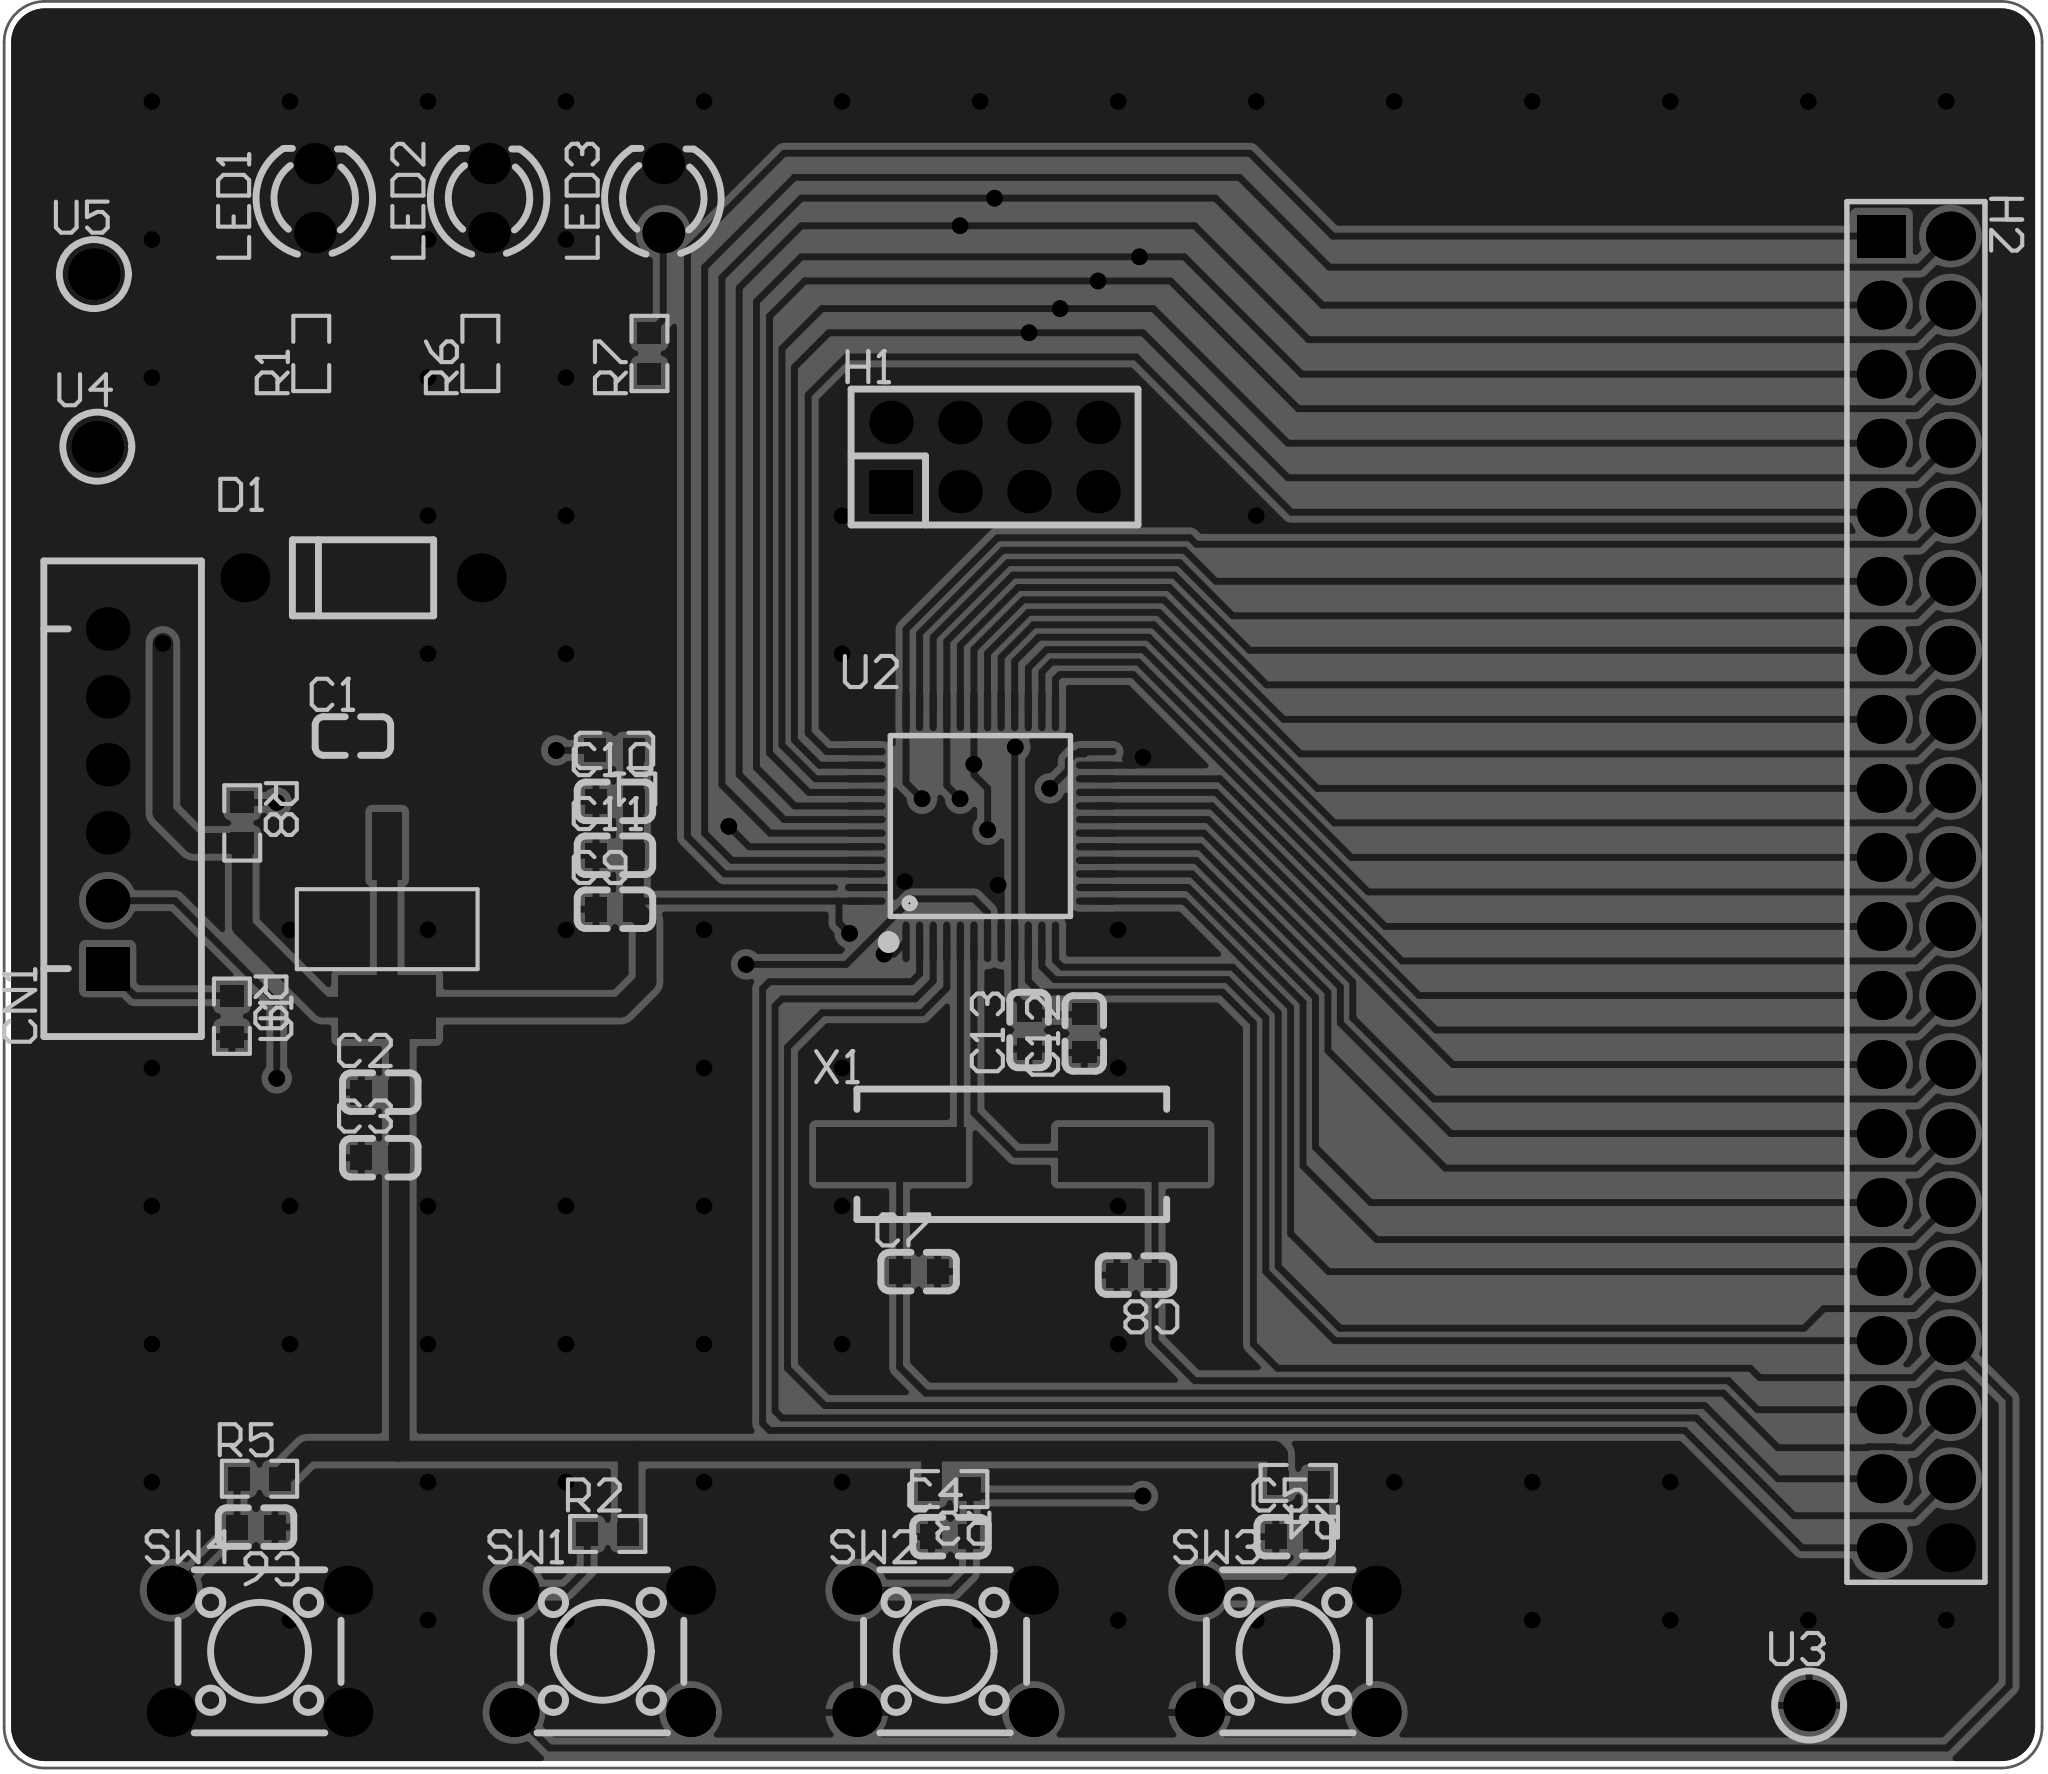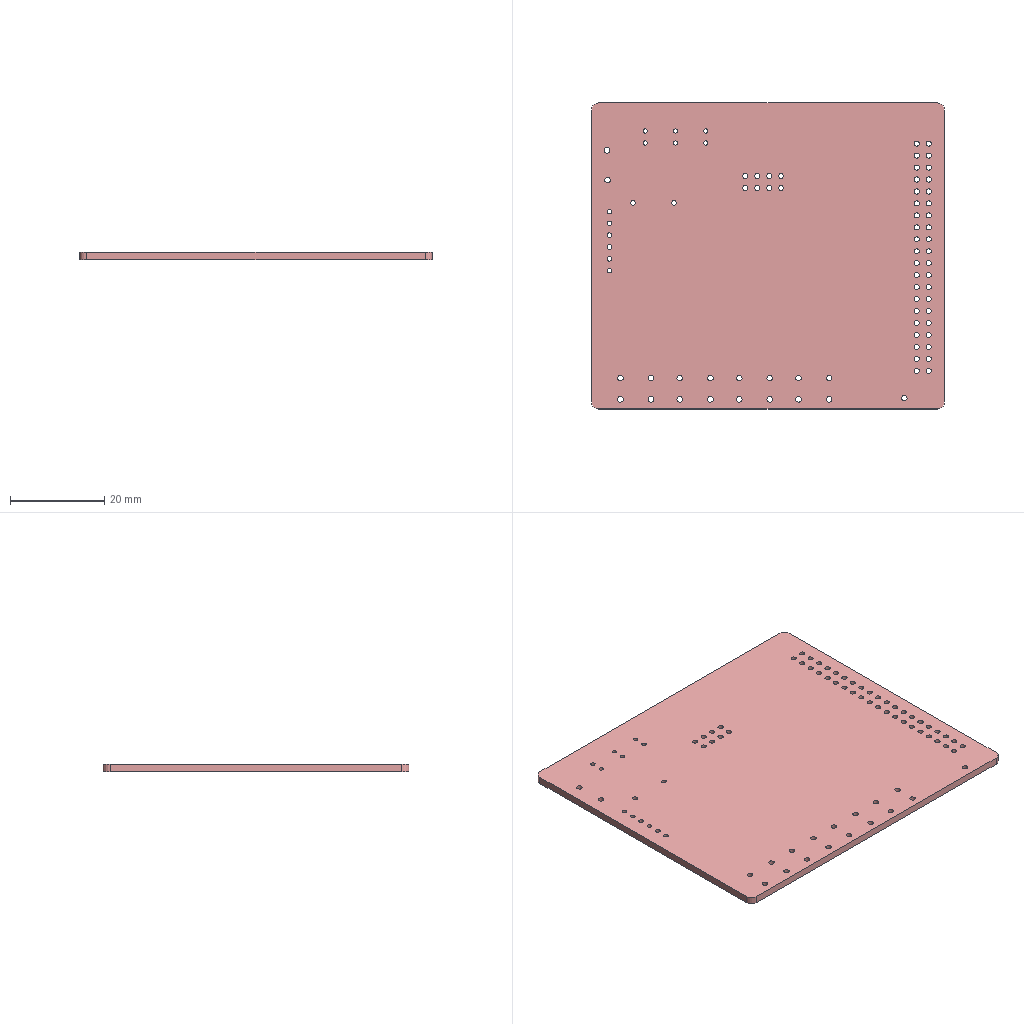Circuit board layout | Altium Designer | box 75 x 65 x 1.6 mm
Layer stack:
# Altium Designer layer stack of  (unit mm; dielectric type: 0 none, 1 core, 2 prepreg, 3 surface material)
index,name,kind,layer,copper_thickness_mm,dielectric_type,dielectric_thickness_mm,dielectric_material,dielectric_constant
0,Top Paste Mask Layer,other,,,,,,
1,Top Silkscreen Layer,other,,,,,,
2,Top Solder Mask Layer,dielectric,,,3,0.01,,3.3
3,Top Layer,copper,Top Layer,0.035,,,,
4,Dielectric1,dielectric,,,3,1.51,FR4,4.5
5,Bottom Layer,copper,Bottom Layer,0.035,,,,
6,Bottom Solder Mask Layer,dielectric,,,3,0.01,,3.3
7,Bottom Silkscreen Layer,other,,,,,,
8,Bottom Paste Mask Layer,other,,,,,,
# drill layer pairs: low layer,high layer
drill_pair,Top Layer,Bottom Layer
Part placement:
Designator,Comment,Layer,Footprint,Center-X(mm),Center-Y(mm),Rotation
C1,47uF,TopLayer,C0603,96.275,119.528,0
C2,47uF,TopLayer,C0603,97.282,106.426,0
C3,100nF,TopLayer,C0603,97.282,104.013,0
C4,100nF,TopLayer,C0603,118.266,90.07,0
C5,100nF,TopLayer,C0603,130.937,90.07,0
C6,100nF,TopLayer,C0603,92.71,90.424,180
C7,22pF,TopLayer,C0603,117.094,99.822,0
C8,22pF,TopLayer,C0603,125.095,99.695,180
C9,100nF,TopLayer,C0603,105.918,113.157,0
C10,100nF,TopLayer,C0603,105.918,117.126,0
C11,100nF,TopLayer,C0603,105.918,115.141,0
C12,1uF,TopLayer,C0603,123.19,108.585,90
C13,10nF,TopLayer,C0603,121.158,108.712,90
CN1,XH-6A,TopLayer,CONN-TH_6P-P2.50_XH-6A,87.249,117.221,90
D1,,TopLayer,DO_1N4007,96.647,125.349,0
H1,A2541HWV-2x4P,TopLayer,HDR-TH_8P-P2.54-V-F-R2-C4-S2.54-1,119.888,129.794,0
H2,2.54mm 2*20P straight pin header,TopLayer,HDR-TH_40P-P2.54-V-M-R2-C20-S2.54,153.797,113.792,270
L1,CBG160808U000T,TopLayer,L0603,105.901,118.999,180
LED1,,TopLayer,LED_TH-3mm,94.869,139.319,90
LED2,,TopLayer,LED_TH-3mm,101.282,139.319,90
LED3,,TopLayer,LED_TH-3mm,107.696,139.319,90
R1,1K,TopLayer,R0603,94.742,133.604,90
R2,10K,TopLayer,R0603,105.651,90.17,0
R3,10K,TopLayer,R0603,118.237,91.821,180
R4,10K,TopLayer,R0603,131.064,92.048,180
R5,10K,TopLayer,R0603,92.837,92.202,0
R6,330,TopLayer,R0603,100.965,133.604,90
R7,330,TopLayer,R0603,107.188,133.604,90
R8,10K,TopLayer,R0603,92.202,116.332,270
R9,10K,TopLayer,R0603,91.821,109.22,270
SW1,TS-1095-A5B2-D1,TopLayer,SW-TH_4P-L6.0-W6.0-P4.50-LS6.5,105.452,85.852,0
SW2,TS-1095-A5B2-D1,TopLayer,SW-TH_4P-L6.0-W6.0-P4.50-LS6.5,118.068,85.852,0
SW3,TS-1095-A5B2-D1,TopLayer,SW-TH_4P-L6.0-W6.0-P4.50-LS6.5,130.683,85.852,0
SW4,TS-1095-A5B2-D1,TopLayer,SW-TH_4P-L6.0-W6.0-P4.50-LS6.5,92.837,85.852,0
U1,AMS1117-3.3,TopLayer,SOT-223-3_L6.5-W3.4-P2.30-LS7.0-BR,97.536,112.522,90
U2,GD32E230C8T6,TopLayer,LQFP-48_L7.0-W7.0-P0.50-LS9.0-BL,119.38,116.205,0
U3,RH-5000,TopLayer,TEST-TH_BD2.54-P1.4_RED,149.868,83.859,0
U4,RH-5000,TopLayer,TEST-TH_BD2.54-P1.4_RED,86.868,130.175,0
U5,RH-5000,TopLayer,TEST-TH_BD2.54-P1.4_RED,86.741,136.525,0
X1,8MHz,TopLayer,CRYSTAL-SMD_L11.5-W4.8-LS12.7,120.523,104.14,0
Pad and via stacks:
# Altium Designer via and pad stacks of  (unit mm). Each distinct definition once, with the count of objects using it.
# via: kind,start_layer,end_layer,hole_mm,diameter_mm,mode(0 simple;1 top-mid-bottom;2 full stack),diameter_per_layer,count,example_net
# pad: kind,layer,hole_mm,hole_type(0 round;1 square;2 slot),plating,top_size,top_shape(1 round;2 rect;3 octagon;9 rounded rect),mid_size,bottom_size,mode,footprint,size_per_layer,count,example
pad,Top Layer,0,0,plated,0.8x0.9,2,0.8x0.9,0.8x0.9,0,C0603,,26,C1.2
pad,Top Layer,0,0,plated,0.8x0.864,2,0.8x0.864,0.8x0.864,0,L0603,,2,L1.1
pad,Top Layer,0,0,plated,0.8065x0.864,2,0.8065x0.864,0.8065x0.864,0,R0603,,18,R1.2
pad,Top Layer,0,0,plated,2.5x1.1,2,2.5x1.1,2.5x1.1,0,SOT-223-3_L6.5-W3.4-P2.30-LS7.0-BR,,3,U1.1
pad,Top Layer,0,0,plated,2.34x3.6,2,2.34x3.6,2.34x3.6,0,SOT-223-3_L6.5-W3.4-P2.30-LS7.0-BR,,1,U1.4
pad,Top Layer,0,0,plated,0.27x1.5,1,0.27x1.5,0.27x1.5,0,LQFP-48_L7.0-W7.0-P0.50-LS9.0-BL,,24,U2.1
pad,Top Layer,0,0,plated,1.5x0.27,1,1.5x0.27,1.5x0.27,0,LQFP-48_L7.0-W7.0-P0.50-LS9.0-BL,,24,U2.13
pad,Top Layer,0,0,plated,5.5x2,2,5.5x2,5.5x2,0,CRYSTAL-SMD_L11.5-W4.8-LS12.7,,2,X1.2
pad,Multi-Layer,1,0,plated,1.6x1.6,2,1.6x1.6,1.6x1.6,0,CONN-TH_6P-P2.50_XH-6A,,1,CN1.1
pad,Multi-Layer,1,0,plated,1.6x1.6,1,1.6x1.6,1.6x1.6,0,CONN-TH_6P-P2.50_XH-6A,,5,CN1.2
pad,Multi-Layer,1,0,plated,1.8x1.8,1,1.8x1.8,1.8x1.8,0,DO_1N4007,,2,D1.1
pad,Multi-Layer,1.1,0,plated,1.6x1.6,2,1.6x1.6,1.6x1.6,0,HDR-TH_8P-P2.54-V-F-R2-C4-S2.54-1,,1,H1.1
pad,Multi-Layer,1.1,0,plated,1.6x1.6,1,1.6x1.6,1.6x1.6,0,HDR-TH_8P-P2.54-V-F-R2-C4-S2.54-1,,7,H1.2
pad,Multi-Layer,1.1,0,plated,1.575x1.8,2,1.575x1.8,1.575x1.8,0,HDR-TH_40P-P2.54-V-M-R2-C20-S2.54,,1,H2.1
pad,Multi-Layer,1.1,0,plated,1.8x1.8,1,1.8x1.8,1.8x1.8,0,HDR-TH_40P-P2.54-V-M-R2-C20-S2.54,,39,H2.2
pad,Multi-Layer,0.9144,0,plated,1.524x1.524,1,1.524x1.524,1.524x1.524,0,LED_TH-3mm,,6,LED1.1
pad,Multi-Layer,1.2,0,plated,1.8x1.8,1,1.8x1.8,1.8x1.8,0,SW-TH_4P-L6.0-W6.0-P4.50-LS6.5,,16,SW1.1
pad,Multi-Layer,1.2,0,plated,1.9x1.9,1,1.9x1.9,1.9x1.9,0,TEST-TH_BD2.54-P1.4_RED,,3,U3.1
via,Top Layer,Bottom Layer,0.3048,0.61,0,,92,PB6
Copper pours:
name,layer,net,type(0 solid;1 hatched;2 none)
Top Layer-GND,Top Layer,GND,0
Bottom Layer-GND,Bottom Layer,GND,0